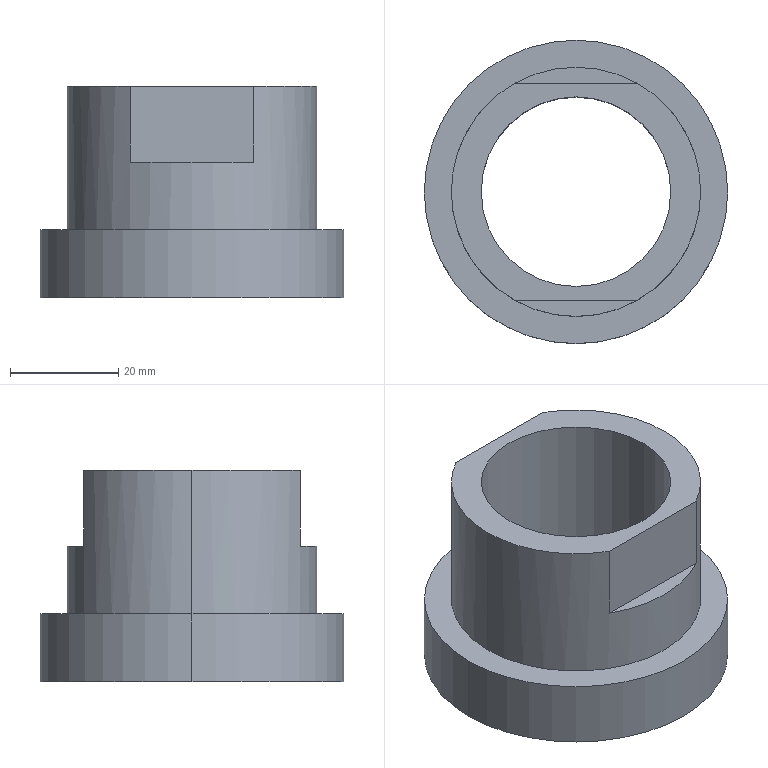Part | STEP file | DAU NOI XY LANH 125 | 1 solid | 13 faces | box 56 x 56 x 39 mm | volume 36016 mm3 | plane 7 | cylinder 6 | commonest cylinder face diameters 35 x2 46 x2 56 x2
STEP:
#1=CARTESIAN_POINT('',(0.,0.,0.));
#2=DIRECTION('',(0.,0.,1.));
#3=DIRECTION('',(1.,0.,0.));
#4=AXIS2_PLACEMENT_3D('',#1,#2,#3);
#5=CARTESIAN_POINT('',(-17.5,0.,39.));
#6=VERTEX_POINT('',#5);
#7=CARTESIAN_POINT('',(-17.5,0.,0.));
#8=VERTEX_POINT('',#7);
#9=CARTESIAN_POINT('',(-17.5,0.,39.));
#10=DIRECTION('',(0.,0.,-1.));
#11=VECTOR('',#10,1.);
#12=LINE('',#9,#11);
#13=CARTESIAN_POINT('',(0.,0.,39.));
#14=DIRECTION('',(0.,0.,-1.));
#15=DIRECTION('',(-1.,0.,0.));
#16=AXIS2_PLACEMENT_3D('',#13,#14,#15);
#17=CYLINDRICAL_SURFACE('',#16,17.5);
#18=CARTESIAN_POINT('',(6.283,0.));
#19=DIRECTION('',(0.,1.));
#20=VECTOR('',#19,1.);
#21=LINE('',#18,#20);
#22=(GEOMETRIC_REPRESENTATION_CONTEXT(2)PARAMETRIC_REPRESENTATION_CONTEXT()REPRESENTATION_CONTEXT('',''));
#23=DEFINITIONAL_REPRESENTATION('',(#21),#22);
#24=PCURVE('',#17,#23);
#25=CARTESIAN_POINT('',(0.,0.,39.));
#26=DIRECTION('',(0.,0.,-1.));
#27=DIRECTION('',(-1.,0.,0.));
#28=AXIS2_PLACEMENT_3D('',#25,#26,#27);
#29=CYLINDRICAL_SURFACE('',#28,17.5);
#30=CARTESIAN_POINT('',(0.,0.));
#31=DIRECTION('',(0.,1.));
#32=VECTOR('',#31,1.);
#33=LINE('',#30,#32);
#34=(GEOMETRIC_REPRESENTATION_CONTEXT(2)PARAMETRIC_REPRESENTATION_CONTEXT()REPRESENTATION_CONTEXT('',''));
#35=DEFINITIONAL_REPRESENTATION('',(#33),#34);
#36=PCURVE('',#29,#35);
#37=SURFACE_CURVE('',#12,(#24,#36),.PCURVE_S1.);
#38=EDGE_CURVE('',#6,#8,#37,.T.);
#39=ORIENTED_EDGE('',*,*,#38,.T.);
#40=CARTESIAN_POINT('',(17.5,0.,0.));
#41=VERTEX_POINT('',#40);
#42=CARTESIAN_POINT('',(0.,0.,0.));
#43=DIRECTION('',(0.,0.,1.));
#44=DIRECTION('',(-1.,0.,0.));
#45=AXIS2_PLACEMENT_3D('',#42,#43,#44);
#46=CIRCLE('',#45,17.5);
#47=CARTESIAN_POINT('',(6.283,39.));
#48=DIRECTION('',(-1.,0.));
#49=VECTOR('',#48,1.);
#50=LINE('',#47,#49);
#51=(GEOMETRIC_REPRESENTATION_CONTEXT(2)PARAMETRIC_REPRESENTATION_CONTEXT()REPRESENTATION_CONTEXT('',''));
#52=DEFINITIONAL_REPRESENTATION('',(#50),#51);
#53=PCURVE('',#17,#52);
#54=CARTESIAN_POINT('',(0.,0.,0.));
#55=DIRECTION('',(0.,0.,-1.));
#56=DIRECTION('',(-1.,0.,0.));
#57=AXIS2_PLACEMENT_3D('',#54,#55,#56);
#58=PLANE('',#57);
#59=CARTESIAN_POINT('',(17.5,0.));
#60=CARTESIAN_POINT('',(17.5,-30.311));
#61=CARTESIAN_POINT('',(-8.75,-15.155));
#62=CARTESIAN_POINT('',(-35.,0.));
#63=CARTESIAN_POINT('',(-8.75,15.155));
#64=CARTESIAN_POINT('',(17.5,30.311));
#65=CARTESIAN_POINT('',(17.5,0.));
#66=(BOUNDED_CURVE()B_SPLINE_CURVE(2,(#59,#60,#61,#62,#63,#64,#65),.UNSPECIFIED.,.T.,.F.)B_SPLINE_CURVE_WITH_KNOTS((1,2,2,2,2,1),(-2.094,0.,2.094,4.189,6.283,8.378),.UNSPECIFIED.)CURVE()GEOMETRIC_REPRESENTATION_ITEM()RATIONAL_B_SPLINE_CURVE((1.,0.5,1.,0.5,1.,0.5,1.))REPRESENTATION_ITEM(''));
#67=(GEOMETRIC_REPRESENTATION_CONTEXT(2)PARAMETRIC_REPRESENTATION_CONTEXT()REPRESENTATION_CONTEXT('',''));
#68=DEFINITIONAL_REPRESENTATION('',(#66),#67);
#69=PCURVE('',#58,#68);
#70=SURFACE_CURVE('',#46,(#53,#69),.PCURVE_S1.);
#71=EDGE_CURVE('',#8,#41,#70,.T.);
#72=ORIENTED_EDGE('',*,*,#71,.T.);
#73=CARTESIAN_POINT('',(17.5,0.,39.));
#74=VERTEX_POINT('',#73);
#75=CARTESIAN_POINT('',(17.5,0.,39.));
#76=DIRECTION('',(0.,0.,-1.));
#77=VECTOR('',#76,1.);
#78=LINE('',#75,#77);
#79=CARTESIAN_POINT('',(3.142,0.));
#80=DIRECTION('',(0.,1.));
#81=VECTOR('',#80,1.);
#82=LINE('',#79,#81);
#83=(GEOMETRIC_REPRESENTATION_CONTEXT(2)PARAMETRIC_REPRESENTATION_CONTEXT()REPRESENTATION_CONTEXT('',''));
#84=DEFINITIONAL_REPRESENTATION('',(#82),#83);
#85=PCURVE('',#17,#84);
#86=CARTESIAN_POINT('',(3.142,0.));
#87=DIRECTION('',(0.,1.));
#88=VECTOR('',#87,1.);
#89=LINE('',#86,#88);
#90=(GEOMETRIC_REPRESENTATION_CONTEXT(2)PARAMETRIC_REPRESENTATION_CONTEXT()REPRESENTATION_CONTEXT('',''));
#91=DEFINITIONAL_REPRESENTATION('',(#89),#90);
#92=PCURVE('',#29,#91);
#93=SURFACE_CURVE('',#78,(#85,#92),.PCURVE_S1.);
#94=EDGE_CURVE('',#74,#41,#93,.T.);
#95=ORIENTED_EDGE('',*,*,#94,.F.);
#96=CARTESIAN_POINT('',(0.,0.,39.));
#97=DIRECTION('',(0.,0.,-1.));
#98=DIRECTION('',(-1.,0.,0.));
#99=AXIS2_PLACEMENT_3D('',#96,#97,#98);
#100=CIRCLE('',#99,17.5);
#101=CARTESIAN_POINT('',(0.,0.));
#102=DIRECTION('',(1.,0.));
#103=VECTOR('',#102,1.);
#104=LINE('',#101,#103);
#105=(GEOMETRIC_REPRESENTATION_CONTEXT(2)PARAMETRIC_REPRESENTATION_CONTEXT()REPRESENTATION_CONTEXT('',''));
#106=DEFINITIONAL_REPRESENTATION('',(#104),#105);
#107=PCURVE('',#17,#106);
#108=CARTESIAN_POINT('',(0.,0.,39.));
#109=DIRECTION('',(0.,0.,-1.));
#110=DIRECTION('',(-1.,0.,0.));
#111=AXIS2_PLACEMENT_3D('',#108,#109,#110);
#112=PLANE('',#111);
#113=CARTESIAN_POINT('',(0.,0.));
#114=DIRECTION('',(1.,0.));
#115=AXIS2_PLACEMENT_2D('',#113,#114);
#116=CIRCLE('',#115,17.5);
#117=(GEOMETRIC_REPRESENTATION_CONTEXT(2)PARAMETRIC_REPRESENTATION_CONTEXT()REPRESENTATION_CONTEXT('',''));
#118=DEFINITIONAL_REPRESENTATION('',(#116),#117);
#119=PCURVE('',#112,#118);
#120=SURFACE_CURVE('',#100,(#107,#119),.PCURVE_S1.);
#121=EDGE_CURVE('',#74,#6,#120,.T.);
#122=ORIENTED_EDGE('',*,*,#121,.T.);
#123=EDGE_LOOP('',(#39,#72,#95,#122));
#124=FACE_BOUND('',#123,.F.);
#125=ADVANCED_FACE('',(#124),#17,.F.);
#126=CARTESIAN_POINT('',(23.,0.,12.5));
#127=VERTEX_POINT('',#126);
#128=CARTESIAN_POINT('',(-23.,0.,12.5));
#129=VERTEX_POINT('',#128);
#130=CARTESIAN_POINT('',(0.,0.,12.5));
#131=DIRECTION('',(0.,0.,1.));
#132=DIRECTION('',(1.,0.,0.));
#133=AXIS2_PLACEMENT_3D('',#130,#131,#132);
#134=CIRCLE('',#133,23.);
#135=CARTESIAN_POINT('',(0.,0.,12.5));
#136=DIRECTION('',(0.,0.,1.));
#137=DIRECTION('',(1.,0.,0.));
#138=AXIS2_PLACEMENT_3D('',#135,#136,#137);
#139=CYLINDRICAL_SURFACE('',#138,23.);
#140=CARTESIAN_POINT('',(0.,0.));
#141=DIRECTION('',(1.,0.));
#142=VECTOR('',#141,1.);
#143=LINE('',#140,#142);
#144=(GEOMETRIC_REPRESENTATION_CONTEXT(2)PARAMETRIC_REPRESENTATION_CONTEXT()REPRESENTATION_CONTEXT('',''));
#145=DEFINITIONAL_REPRESENTATION('',(#143),#144);
#146=PCURVE('',#139,#145);
#147=CARTESIAN_POINT('',(0.,0.,12.5));
#148=DIRECTION('',(0.,0.,-1.));
#149=DIRECTION('',(-1.,0.,0.));
#150=AXIS2_PLACEMENT_3D('',#147,#148,#149);
#151=PLANE('',#150);
#152=CARTESIAN_POINT('',(-23.,0.));
#153=CARTESIAN_POINT('',(-23.,39.837));
#154=CARTESIAN_POINT('',(11.5,19.919));
#155=CARTESIAN_POINT('',(46.,0.));
#156=CARTESIAN_POINT('',(11.5,-19.919));
#157=CARTESIAN_POINT('',(-23.,-39.837));
#158=CARTESIAN_POINT('',(-23.,0.));
#159=(BOUNDED_CURVE()B_SPLINE_CURVE(2,(#152,#153,#154,#155,#156,#157,#158),.UNSPECIFIED.,.T.,.F.)B_SPLINE_CURVE_WITH_KNOTS((1,2,2,2,2,1),(-2.094,0.,2.094,4.189,6.283,8.378),.UNSPECIFIED.)CURVE()GEOMETRIC_REPRESENTATION_ITEM()RATIONAL_B_SPLINE_CURVE((1.,0.5,1.,0.5,1.,0.5,1.))REPRESENTATION_ITEM(''));
#160=(GEOMETRIC_REPRESENTATION_CONTEXT(2)PARAMETRIC_REPRESENTATION_CONTEXT()REPRESENTATION_CONTEXT('',''));
#161=DEFINITIONAL_REPRESENTATION('',(#159),#160);
#162=PCURVE('',#151,#161);
#163=SURFACE_CURVE('',#134,(#146,#162),.PCURVE_S1.);
#164=EDGE_CURVE('',#127,#129,#163,.T.);
#165=ORIENTED_EDGE('',*,*,#164,.T.);
#166=CARTESIAN_POINT('',(-23.,0.,39.));
#167=VERTEX_POINT('',#166);
#168=CARTESIAN_POINT('',(-23.,0.,12.5));
#169=DIRECTION('',(0.,0.,1.));
#170=VECTOR('',#169,1.);
#171=LINE('',#168,#170);
#172=CARTESIAN_POINT('',(3.142,0.));
#173=DIRECTION('',(0.,1.));
#174=VECTOR('',#173,1.);
#175=LINE('',#172,#174);
#176=(GEOMETRIC_REPRESENTATION_CONTEXT(2)PARAMETRIC_REPRESENTATION_CONTEXT()REPRESENTATION_CONTEXT('',''));
#177=DEFINITIONAL_REPRESENTATION('',(#175),#176);
#178=PCURVE('',#139,#177);
#179=CARTESIAN_POINT('',(0.,0.,12.5));
#180=DIRECTION('',(0.,0.,1.));
#181=DIRECTION('',(1.,0.,0.));
#182=AXIS2_PLACEMENT_3D('',#179,#180,#181);
#183=CYLINDRICAL_SURFACE('',#182,23.);
#184=CARTESIAN_POINT('',(3.142,0.));
#185=DIRECTION('',(0.,1.));
#186=VECTOR('',#185,1.);
#187=LINE('',#184,#186);
#188=(GEOMETRIC_REPRESENTATION_CONTEXT(2)PARAMETRIC_REPRESENTATION_CONTEXT()REPRESENTATION_CONTEXT('',''));
#189=DEFINITIONAL_REPRESENTATION('',(#187),#188);
#190=PCURVE('',#183,#189);
#191=SURFACE_CURVE('',#171,(#178,#190),.PCURVE_S1.);
#192=EDGE_CURVE('',#129,#167,#191,.T.);
#193=ORIENTED_EDGE('',*,*,#192,.T.);
#194=CARTESIAN_POINT('',(-11.358,20.,39.));
#195=VERTEX_POINT('',#194);
#196=CARTESIAN_POINT('',(0.,0.,39.));
#197=DIRECTION('',(0.,0.,-1.));
#198=DIRECTION('',(1.,0.,0.));
#199=AXIS2_PLACEMENT_3D('',#196,#197,#198);
#200=CIRCLE('',#199,23.);
#201=CARTESIAN_POINT('',(6.283,26.5));
#202=DIRECTION('',(-1.,0.));
#203=VECTOR('',#202,1.);
#204=LINE('',#201,#203);
#205=(GEOMETRIC_REPRESENTATION_CONTEXT(2)PARAMETRIC_REPRESENTATION_CONTEXT()REPRESENTATION_CONTEXT('',''));
#206=DEFINITIONAL_REPRESENTATION('',(#204),#205);
#207=PCURVE('',#139,#206);
#208=CARTESIAN_POINT('',(0.,0.));
#209=DIRECTION('',(-1.,0.));
#210=AXIS2_PLACEMENT_2D('',#208,#209);
#211=CIRCLE('',#210,23.);
#212=(GEOMETRIC_REPRESENTATION_CONTEXT(2)PARAMETRIC_REPRESENTATION_CONTEXT()REPRESENTATION_CONTEXT('',''));
#213=DEFINITIONAL_REPRESENTATION('',(#211),#212);
#214=PCURVE('',#112,#213);
#215=SURFACE_CURVE('',#200,(#207,#214),.PCURVE_S1.);
#216=EDGE_CURVE('',#167,#195,#215,.T.);
#217=ORIENTED_EDGE('',*,*,#216,.T.);
#218=CARTESIAN_POINT('',(-11.358,20.,25.));
#219=VERTEX_POINT('',#218);
#220=CARTESIAN_POINT('',(-11.358,20.,12.5));
#221=DIRECTION('',(0.,0.,-1.));
#222=VECTOR('',#221,1.);
#223=LINE('',#220,#222);
#224=CARTESIAN_POINT('',(2.087,0.));
#225=DIRECTION('',(0.,-1.));
#226=VECTOR('',#225,1.);
#227=LINE('',#224,#226);
#228=(GEOMETRIC_REPRESENTATION_CONTEXT(2)PARAMETRIC_REPRESENTATION_CONTEXT()REPRESENTATION_CONTEXT('',''));
#229=DEFINITIONAL_REPRESENTATION('',(#227),#228);
#230=PCURVE('',#139,#229);
#231=CARTESIAN_POINT('',(-15.,20.,39.));
#232=DIRECTION('',(0.,-1.,0.));
#233=DIRECTION('',(0.,0.,-1.));
#234=AXIS2_PLACEMENT_3D('',#231,#232,#233);
#235=PLANE('',#234);
#236=CARTESIAN_POINT('',(26.5,3.642));
#237=DIRECTION('',(1.,0.));
#238=VECTOR('',#237,1.);
#239=LINE('',#236,#238);
#240=(GEOMETRIC_REPRESENTATION_CONTEXT(2)PARAMETRIC_REPRESENTATION_CONTEXT()REPRESENTATION_CONTEXT('',''));
#241=DEFINITIONAL_REPRESENTATION('',(#239),#240);
#242=PCURVE('',#235,#241);
#243=SURFACE_CURVE('',#223,(#230,#242),.PCURVE_S1.);
#244=EDGE_CURVE('',#195,#219,#243,.T.);
#245=ORIENTED_EDGE('',*,*,#244,.T.);
#246=CARTESIAN_POINT('',(11.358,20.,25.));
#247=VERTEX_POINT('',#246);
#248=CARTESIAN_POINT('',(0.,0.,25.));
#249=DIRECTION('',(0.,0.,-1.));
#250=DIRECTION('',(1.,0.,0.));
#251=AXIS2_PLACEMENT_3D('',#248,#249,#250);
#252=CIRCLE('',#251,23.);
#253=CARTESIAN_POINT('',(6.283,12.5));
#254=DIRECTION('',(-1.,0.));
#255=VECTOR('',#254,1.);
#256=LINE('',#253,#255);
#257=(GEOMETRIC_REPRESENTATION_CONTEXT(2)PARAMETRIC_REPRESENTATION_CONTEXT()REPRESENTATION_CONTEXT('',''));
#258=DEFINITIONAL_REPRESENTATION('',(#256),#257);
#259=PCURVE('',#139,#258);
#260=CARTESIAN_POINT('',(0.,25.,25.));
#261=DIRECTION('',(0.,0.,1.));
#262=DIRECTION('',(1.,0.,0.));
#263=AXIS2_PLACEMENT_3D('',#260,#261,#262);
#264=PLANE('',#263);
#265=CARTESIAN_POINT('',(23.,-25.));
#266=CARTESIAN_POINT('',(23.,-64.837));
#267=CARTESIAN_POINT('',(-11.5,-44.919));
#268=CARTESIAN_POINT('',(-46.,-25.));
#269=CARTESIAN_POINT('',(-11.5,-5.081));
#270=CARTESIAN_POINT('',(23.,14.837));
#271=CARTESIAN_POINT('',(23.,-25.));
#272=(BOUNDED_CURVE()B_SPLINE_CURVE(2,(#265,#266,#267,#268,#269,#270,#271),.UNSPECIFIED.,.T.,.F.)B_SPLINE_CURVE_WITH_KNOTS((1,2,2,2,2,1),(-2.094,0.,2.094,4.189,6.283,8.378),.UNSPECIFIED.)CURVE()GEOMETRIC_REPRESENTATION_ITEM()RATIONAL_B_SPLINE_CURVE((1.,0.5,1.,0.5,1.,0.5,1.))REPRESENTATION_ITEM(''));
#273=(GEOMETRIC_REPRESENTATION_CONTEXT(2)PARAMETRIC_REPRESENTATION_CONTEXT()REPRESENTATION_CONTEXT('',''));
#274=DEFINITIONAL_REPRESENTATION('',(#272),#273);
#275=PCURVE('',#264,#274);
#276=SURFACE_CURVE('',#252,(#259,#275),.PCURVE_S1.);
#277=EDGE_CURVE('',#219,#247,#276,.T.);
#278=ORIENTED_EDGE('',*,*,#277,.T.);
#279=CARTESIAN_POINT('',(11.358,20.,39.));
#280=VERTEX_POINT('',#279);
#281=CARTESIAN_POINT('',(11.358,20.,12.5));
#282=DIRECTION('',(0.,0.,1.));
#283=VECTOR('',#282,1.);
#284=LINE('',#281,#283);
#285=CARTESIAN_POINT('',(1.054,0.));
#286=DIRECTION('',(0.,1.));
#287=VECTOR('',#286,1.);
#288=LINE('',#285,#287);
#289=(GEOMETRIC_REPRESENTATION_CONTEXT(2)PARAMETRIC_REPRESENTATION_CONTEXT()REPRESENTATION_CONTEXT('',''));
#290=DEFINITIONAL_REPRESENTATION('',(#288),#289);
#291=PCURVE('',#139,#290);
#292=CARTESIAN_POINT('',(26.5,26.358));
#293=DIRECTION('',(-1.,0.));
#294=VECTOR('',#293,1.);
#295=LINE('',#292,#294);
#296=(GEOMETRIC_REPRESENTATION_CONTEXT(2)PARAMETRIC_REPRESENTATION_CONTEXT()REPRESENTATION_CONTEXT('',''));
#297=DEFINITIONAL_REPRESENTATION('',(#295),#296);
#298=PCURVE('',#235,#297);
#299=SURFACE_CURVE('',#284,(#291,#298),.PCURVE_S1.);
#300=EDGE_CURVE('',#247,#280,#299,.T.);
#301=ORIENTED_EDGE('',*,*,#300,.T.);
#302=CARTESIAN_POINT('',(23.,0.,39.));
#303=VERTEX_POINT('',#302);
#304=CARTESIAN_POINT('',(0.,0.,39.));
#305=DIRECTION('',(0.,0.,-1.));
#306=DIRECTION('',(1.,0.,0.));
#307=AXIS2_PLACEMENT_3D('',#304,#305,#306);
#308=CIRCLE('',#307,23.);
#309=CARTESIAN_POINT('',(6.283,26.5));
#310=DIRECTION('',(-1.,0.));
#311=VECTOR('',#310,1.);
#312=LINE('',#309,#311);
#313=(GEOMETRIC_REPRESENTATION_CONTEXT(2)PARAMETRIC_REPRESENTATION_CONTEXT()REPRESENTATION_CONTEXT('',''));
#314=DEFINITIONAL_REPRESENTATION('',(#312),#313);
#315=PCURVE('',#139,#314);
#316=CARTESIAN_POINT('',(0.,0.));
#317=DIRECTION('',(-1.,0.));
#318=AXIS2_PLACEMENT_2D('',#316,#317);
#319=CIRCLE('',#318,23.);
#320=(GEOMETRIC_REPRESENTATION_CONTEXT(2)PARAMETRIC_REPRESENTATION_CONTEXT()REPRESENTATION_CONTEXT('',''));
#321=DEFINITIONAL_REPRESENTATION('',(#319),#320);
#322=PCURVE('',#112,#321);
#323=SURFACE_CURVE('',#308,(#315,#322),.PCURVE_S1.);
#324=EDGE_CURVE('',#280,#303,#323,.T.);
#325=ORIENTED_EDGE('',*,*,#324,.T.);
#326=CARTESIAN_POINT('',(23.,0.,12.5));
#327=DIRECTION('',(0.,0.,1.));
#328=VECTOR('',#327,1.);
#329=LINE('',#326,#328);
#330=CARTESIAN_POINT('',(0.,0.));
#331=DIRECTION('',(0.,1.));
#332=VECTOR('',#331,1.);
#333=LINE('',#330,#332);
#334=(GEOMETRIC_REPRESENTATION_CONTEXT(2)PARAMETRIC_REPRESENTATION_CONTEXT()REPRESENTATION_CONTEXT('',''));
#335=DEFINITIONAL_REPRESENTATION('',(#333),#334);
#336=PCURVE('',#139,#335);
#337=CARTESIAN_POINT('',(6.283,0.));
#338=DIRECTION('',(0.,1.));
#339=VECTOR('',#338,1.);
#340=LINE('',#337,#339);
#341=(GEOMETRIC_REPRESENTATION_CONTEXT(2)PARAMETRIC_REPRESENTATION_CONTEXT()REPRESENTATION_CONTEXT('',''));
#342=DEFINITIONAL_REPRESENTATION('',(#340),#341);
#343=PCURVE('',#183,#342);
#344=SURFACE_CURVE('',#329,(#336,#343),.PCURVE_S1.);
#345=EDGE_CURVE('',#127,#303,#344,.T.);
#346=ORIENTED_EDGE('',*,*,#345,.F.);
#347=EDGE_LOOP('',(#165,#193,#217,#245,#278,#301,#325,#346));
#348=FACE_BOUND('',#347,.T.);
#349=ADVANCED_FACE('',(#348),#139,.T.);
#350=CARTESIAN_POINT('',(-28.,0.,0.));
#351=VERTEX_POINT('',#350);
#352=CARTESIAN_POINT('',(28.,0.,0.));
#353=VERTEX_POINT('',#352);
#354=CARTESIAN_POINT('',(0.,0.,0.));
#355=DIRECTION('',(0.,0.,-1.));
#356=DIRECTION('',(1.,0.,0.));
#357=AXIS2_PLACEMENT_3D('',#354,#355,#356);
#358=CIRCLE('',#357,28.);
#359=CARTESIAN_POINT('',(0.,0.,0.));
#360=DIRECTION('',(0.,0.,1.));
#361=DIRECTION('',(1.,0.,0.));
#362=AXIS2_PLACEMENT_3D('',#359,#360,#361);
#363=CYLINDRICAL_SURFACE('',#362,28.);
#364=CARTESIAN_POINT('',(6.283,0.));
#365=DIRECTION('',(-1.,0.));
#366=VECTOR('',#365,1.);
#367=LINE('',#364,#366);
#368=(GEOMETRIC_REPRESENTATION_CONTEXT(2)PARAMETRIC_REPRESENTATION_CONTEXT()REPRESENTATION_CONTEXT('',''));
#369=DEFINITIONAL_REPRESENTATION('',(#367),#368);
#370=PCURVE('',#363,#369);
#371=CARTESIAN_POINT('',(0.,0.));
#372=DIRECTION('',(-1.,0.));
#373=AXIS2_PLACEMENT_2D('',#371,#372);
#374=CIRCLE('',#373,28.);
#375=(GEOMETRIC_REPRESENTATION_CONTEXT(2)PARAMETRIC_REPRESENTATION_CONTEXT()REPRESENTATION_CONTEXT('',''));
#376=DEFINITIONAL_REPRESENTATION('',(#374),#375);
#377=PCURVE('',#58,#376);
#378=SURFACE_CURVE('',#358,(#370,#377),.PCURVE_S1.);
#379=EDGE_CURVE('',#351,#353,#378,.T.);
#380=ORIENTED_EDGE('',*,*,#379,.F.);
#381=CARTESIAN_POINT('',(-28.,0.,12.5));
#382=VERTEX_POINT('',#381);
#383=CARTESIAN_POINT('',(-28.,0.,0.));
#384=DIRECTION('',(0.,0.,1.));
#385=VECTOR('',#384,1.);
#386=LINE('',#383,#385);
#387=CARTESIAN_POINT('',(3.142,0.));
#388=DIRECTION('',(0.,1.));
#389=VECTOR('',#388,1.);
#390=LINE('',#387,#389);
#391=(GEOMETRIC_REPRESENTATION_CONTEXT(2)PARAMETRIC_REPRESENTATION_CONTEXT()REPRESENTATION_CONTEXT('',''));
#392=DEFINITIONAL_REPRESENTATION('',(#390),#391);
#393=PCURVE('',#363,#392);
#394=CARTESIAN_POINT('',(0.,0.,0.));
#395=DIRECTION('',(0.,0.,1.));
#396=DIRECTION('',(1.,0.,0.));
#397=AXIS2_PLACEMENT_3D('',#394,#395,#396);
#398=CYLINDRICAL_SURFACE('',#397,28.);
#399=CARTESIAN_POINT('',(3.142,0.));
#400=DIRECTION('',(0.,1.));
#401=VECTOR('',#400,1.);
#402=LINE('',#399,#401);
#403=(GEOMETRIC_REPRESENTATION_CONTEXT(2)PARAMETRIC_REPRESENTATION_CONTEXT()REPRESENTATION_CONTEXT('',''));
#404=DEFINITIONAL_REPRESENTATION('',(#402),#403);
#405=PCURVE('',#398,#404);
#406=SURFACE_CURVE('',#386,(#393,#405),.PCURVE_S1.);
#407=EDGE_CURVE('',#351,#382,#406,.T.);
#408=ORIENTED_EDGE('',*,*,#407,.T.);
#409=CARTESIAN_POINT('',(28.,0.,12.5));
#410=VERTEX_POINT('',#409);
#411=CARTESIAN_POINT('',(0.,0.,12.5));
#412=DIRECTION('',(0.,0.,-1.));
#413=DIRECTION('',(1.,0.,0.));
#414=AXIS2_PLACEMENT_3D('',#411,#412,#413);
#415=CIRCLE('',#414,28.);
#416=CARTESIAN_POINT('',(6.283,12.5));
#417=DIRECTION('',(-1.,0.));
#418=VECTOR('',#417,1.);
#419=LINE('',#416,#418);
#420=(GEOMETRIC_REPRESENTATION_CONTEXT(2)PARAMETRIC_REPRESENTATION_CONTEXT()REPRESENTATION_CONTEXT('',''));
#421=DEFINITIONAL_REPRESENTATION('',(#419),#420);
#422=PCURVE('',#363,#421);
#423=CARTESIAN_POINT('',(0.,0.));
#424=DIRECTION('',(-1.,0.));
#425=AXIS2_PLACEMENT_2D('',#423,#424);
#426=CIRCLE('',#425,28.);
#427=(GEOMETRIC_REPRESENTATION_CONTEXT(2)PARAMETRIC_REPRESENTATION_CONTEXT()REPRESENTATION_CONTEXT('',''));
#428=DEFINITIONAL_REPRESENTATION('',(#426),#427);
#429=PCURVE('',#151,#428);
#430=SURFACE_CURVE('',#415,(#422,#429),.PCURVE_S1.);
#431=EDGE_CURVE('',#382,#410,#430,.T.);
#432=ORIENTED_EDGE('',*,*,#431,.T.);
#433=CARTESIAN_POINT('',(28.,0.,0.));
#434=DIRECTION('',(0.,0.,1.));
#435=VECTOR('',#434,1.);
#436=LINE('',#433,#435);
#437=CARTESIAN_POINT('',(0.,0.));
#438=DIRECTION('',(0.,1.));
#439=VECTOR('',#438,1.);
#440=LINE('',#437,#439);
#441=(GEOMETRIC_REPRESENTATION_CONTEXT(2)PARAMETRIC_REPRESENTATION_CONTEXT()REPRESENTATION_CONTEXT('',''));
#442=DEFINITIONAL_REPRESENTATION('',(#440),#441);
#443=PCURVE('',#363,#442);
#444=CARTESIAN_POINT('',(6.283,0.));
#445=DIRECTION('',(0.,1.));
#446=VECTOR('',#445,1.);
#447=LINE('',#444,#446);
#448=(GEOMETRIC_REPRESENTATION_CONTEXT(2)PARAMETRIC_REPRESENTATION_CONTEXT()REPRESENTATION_CONTEXT('',''));
#449=DEFINITIONAL_REPRESENTATION('',(#447),#448);
#450=PCURVE('',#398,#449);
#451=SURFACE_CURVE('',#436,(#443,#450),.PCURVE_S1.);
#452=EDGE_CURVE('',#353,#410,#451,.T.);
#453=ORIENTED_EDGE('',*,*,#452,.F.);
#454=EDGE_LOOP('',(#380,#408,#432,#453));
#455=FACE_BOUND('',#454,.T.);
#456=ADVANCED_FACE('',(#455),#363,.T.);
#457=CARTESIAN_POINT('',(0.,0.,0.));
#458=DIRECTION('',(0.,0.,1.));
#459=DIRECTION('',(-1.,0.,0.));
#460=AXIS2_PLACEMENT_3D('',#457,#458,#459);
#461=CIRCLE('',#460,17.5);
#462=CARTESIAN_POINT('',(6.283,39.));
#463=DIRECTION('',(-1.,0.));
#464=VECTOR('',#463,1.);
#465=LINE('',#462,#464);
#466=(GEOMETRIC_REPRESENTATION_CONTEXT(2)PARAMETRIC_REPRESENTATION_CONTEXT()REPRESENTATION_CONTEXT('',''));
#467=DEFINITIONAL_REPRESENTATION('',(#465),#466);
#468=PCURVE('',#29,#467);
#469=CARTESIAN_POINT('',(17.5,0.));
#470=CARTESIAN_POINT('',(17.5,-30.311));
#471=CARTESIAN_POINT('',(-8.75,-15.155));
#472=CARTESIAN_POINT('',(-35.,0.));
#473=CARTESIAN_POINT('',(-8.75,15.155));
#474=CARTESIAN_POINT('',(17.5,30.311));
#475=CARTESIAN_POINT('',(17.5,0.));
#476=(BOUNDED_CURVE()B_SPLINE_CURVE(2,(#469,#470,#471,#472,#473,#474,#475),.UNSPECIFIED.,.T.,.F.)B_SPLINE_CURVE_WITH_KNOTS((1,2,2,2,2,1),(-2.094,0.,2.094,4.189,6.283,8.378),.UNSPECIFIED.)CURVE()GEOMETRIC_REPRESENTATION_ITEM()RATIONAL_B_SPLINE_CURVE((1.,0.5,1.,0.5,1.,0.5,1.))REPRESENTATION_ITEM(''));
#477=(GEOMETRIC_REPRESENTATION_CONTEXT(2)PARAMETRIC_REPRESENTATION_CONTEXT()REPRESENTATION_CONTEXT('',''));
#478=DEFINITIONAL_REPRESENTATION('',(#476),#477);
#479=PCURVE('',#58,#478);
#480=SURFACE_CURVE('',#461,(#468,#479),.PCURVE_S1.);
#481=EDGE_CURVE('',#41,#8,#480,.T.);
#482=ORIENTED_EDGE('',*,*,#481,.T.);
#483=ORIENTED_EDGE('',*,*,#38,.F.);
#484=CARTESIAN_POINT('',(0.,0.,39.));
#485=DIRECTION('',(0.,0.,-1.));
#486=DIRECTION('',(-1.,0.,0.));
#487=AXIS2_PLACEMENT_3D('',#484,#485,#486);
#488=CIRCLE('',#487,17.5);
#489=CARTESIAN_POINT('',(0.,0.));
#490=DIRECTION('',(1.,0.));
#491=VECTOR('',#490,1.);
#492=LINE('',#489,#491);
#493=(GEOMETRIC_REPRESENTATION_CONTEXT(2)PARAMETRIC_REPRESENTATION_CONTEXT()REPRESENTATION_CONTEXT('',''));
#494=DEFINITIONAL_REPRESENTATION('',(#492),#493);
#495=PCURVE('',#29,#494);
#496=CARTESIAN_POINT('',(0.,0.));
#497=DIRECTION('',(1.,0.));
#498=AXIS2_PLACEMENT_2D('',#496,#497);
#499=CIRCLE('',#498,17.5);
#500=(GEOMETRIC_REPRESENTATION_CONTEXT(2)PARAMETRIC_REPRESENTATION_CONTEXT()REPRESENTATION_CONTEXT('',''));
#501=DEFINITIONAL_REPRESENTATION('',(#499),#500);
#502=PCURVE('',#112,#501);
#503=SURFACE_CURVE('',#488,(#495,#502),.PCURVE_S1.);
#504=EDGE_CURVE('',#6,#74,#503,.T.);
#505=ORIENTED_EDGE('',*,*,#504,.T.);
#506=ORIENTED_EDGE('',*,*,#94,.T.);
#507=EDGE_LOOP('',(#482,#483,#505,#506));
#508=FACE_BOUND('',#507,.F.);
#509=ADVANCED_FACE('',(#508),#29,.F.);
#510=ORIENTED_EDGE('',*,*,#504,.T.);
#511=ORIENTED_EDGE('',*,*,#121,.T.);
#512=EDGE_LOOP('',(#510,#511));
#513=FACE_BOUND('',#512,.T.);
#514=ORIENTED_EDGE('',*,*,#324,.F.);
#515=CARTESIAN_POINT('',(0.,20.,39.));
#516=DIRECTION('',(1.,0.,0.));
#517=VECTOR('',#516,1.);
#518=LINE('',#515,#517);
#519=CARTESIAN_POINT('',(0.,20.));
#520=DIRECTION('',(-1.,0.));
#521=VECTOR('',#520,1.);
#522=LINE('',#519,#521);
#523=(GEOMETRIC_REPRESENTATION_CONTEXT(2)PARAMETRIC_REPRESENTATION_CONTEXT()REPRESENTATION_CONTEXT('',''));
#524=DEFINITIONAL_REPRESENTATION('',(#522),#523);
#525=PCURVE('',#112,#524);
#526=CARTESIAN_POINT('',(0.,15.));
#527=DIRECTION('',(0.,1.));
#528=VECTOR('',#527,1.);
#529=LINE('',#526,#528);
#530=(GEOMETRIC_REPRESENTATION_CONTEXT(2)PARAMETRIC_REPRESENTATION_CONTEXT()REPRESENTATION_CONTEXT('',''));
#531=DEFINITIONAL_REPRESENTATION('',(#529),#530);
#532=PCURVE('',#235,#531);
#533=SURFACE_CURVE('',#518,(#525,#532),.PCURVE_S1.);
#534=EDGE_CURVE('',#195,#280,#533,.T.);
#535=ORIENTED_EDGE('',*,*,#534,.F.);
#536=ORIENTED_EDGE('',*,*,#216,.F.);
#537=CARTESIAN_POINT('',(-11.358,-20.,39.));
#538=VERTEX_POINT('',#537);
#539=CARTESIAN_POINT('',(0.,0.,39.));
#540=DIRECTION('',(0.,0.,-1.));
#541=DIRECTION('',(1.,0.,0.));
#542=AXIS2_PLACEMENT_3D('',#539,#540,#541);
#543=CIRCLE('',#542,23.);
#544=CARTESIAN_POINT('',(0.,0.));
#545=DIRECTION('',(-1.,0.));
#546=AXIS2_PLACEMENT_2D('',#544,#545);
#547=CIRCLE('',#546,23.);
#548=(GEOMETRIC_REPRESENTATION_CONTEXT(2)PARAMETRIC_REPRESENTATION_CONTEXT()REPRESENTATION_CONTEXT('',''));
#549=DEFINITIONAL_REPRESENTATION('',(#547),#548);
#550=PCURVE('',#112,#549);
#551=CARTESIAN_POINT('',(6.283,26.5));
#552=DIRECTION('',(-1.,0.));
#553=VECTOR('',#552,1.);
#554=LINE('',#551,#553);
#555=(GEOMETRIC_REPRESENTATION_CONTEXT(2)PARAMETRIC_REPRESENTATION_CONTEXT()REPRESENTATION_CONTEXT('',''));
#556=DEFINITIONAL_REPRESENTATION('',(#554),#555);
#557=PCURVE('',#183,#556);
#558=SURFACE_CURVE('',#543,(#550,#557),.PCURVE_S1.);
#559=EDGE_CURVE('',#538,#167,#558,.T.);
#560=ORIENTED_EDGE('',*,*,#559,.F.);
#561=CARTESIAN_POINT('',(11.358,-20.,39.));
#562=VERTEX_POINT('',#561);
#563=CARTESIAN_POINT('',(0.,-20.,39.));
#564=DIRECTION('',(-1.,0.,0.));
#565=VECTOR('',#564,1.);
#566=LINE('',#563,#565);
#567=CARTESIAN_POINT('',(0.,-20.));
#568=DIRECTION('',(1.,0.));
#569=VECTOR('',#568,1.);
#570=LINE('',#567,#569);
#571=(GEOMETRIC_REPRESENTATION_CONTEXT(2)PARAMETRIC_REPRESENTATION_CONTEXT()REPRESENTATION_CONTEXT('',''));
#572=DEFINITIONAL_REPRESENTATION('',(#570),#571);
#573=PCURVE('',#112,#572);
#574=CARTESIAN_POINT('',(15.,-20.,39.));
#575=DIRECTION('',(0.,1.,0.));
#576=DIRECTION('',(0.,0.,1.));
#577=AXIS2_PLACEMENT_3D('',#574,#575,#576);
#578=PLANE('',#577);
#579=CARTESIAN_POINT('',(0.,-15.));
#580=DIRECTION('',(0.,-1.));
#581=VECTOR('',#580,1.);
#582=LINE('',#579,#581);
#583=(GEOMETRIC_REPRESENTATION_CONTEXT(2)PARAMETRIC_REPRESENTATION_CONTEXT()REPRESENTATION_CONTEXT('',''));
#584=DEFINITIONAL_REPRESENTATION('',(#582),#583);
#585=PCURVE('',#578,#584);
#586=SURFACE_CURVE('',#566,(#573,#585),.PCURVE_S1.);
#587=EDGE_CURVE('',#562,#538,#586,.T.);
#588=ORIENTED_EDGE('',*,*,#587,.F.);
#589=CARTESIAN_POINT('',(0.,0.,39.));
#590=DIRECTION('',(0.,0.,-1.));
#591=DIRECTION('',(1.,0.,0.));
#592=AXIS2_PLACEMENT_3D('',#589,#590,#591);
#593=CIRCLE('',#592,23.);
#594=CARTESIAN_POINT('',(0.,0.));
#595=DIRECTION('',(-1.,0.));
#596=AXIS2_PLACEMENT_2D('',#594,#595);
#597=CIRCLE('',#596,23.);
#598=(GEOMETRIC_REPRESENTATION_CONTEXT(2)PARAMETRIC_REPRESENTATION_CONTEXT()REPRESENTATION_CONTEXT('',''));
#599=DEFINITIONAL_REPRESENTATION('',(#597),#598);
#600=PCURVE('',#112,#599);
#601=CARTESIAN_POINT('',(6.283,26.5));
#602=DIRECTION('',(-1.,0.));
#603=VECTOR('',#602,1.);
#604=LINE('',#601,#603);
#605=(GEOMETRIC_REPRESENTATION_CONTEXT(2)PARAMETRIC_REPRESENTATION_CONTEXT()REPRESENTATION_CONTEXT('',''));
#606=DEFINITIONAL_REPRESENTATION('',(#604),#605);
#607=PCURVE('',#183,#606);
#608=SURFACE_CURVE('',#593,(#600,#607),.PCURVE_S1.);
#609=EDGE_CURVE('',#303,#562,#608,.T.);
#610=ORIENTED_EDGE('',*,*,#609,.F.);
#611=EDGE_LOOP('',(#514,#535,#536,#560,#588,#610));
#612=FACE_BOUND('',#611,.T.);
#613=ADVANCED_FACE('',(#513,#612),#112,.F.);
#614=ORIENTED_EDGE('',*,*,#71,.T.);
#615=ORIENTED_EDGE('',*,*,#481,.T.);
#616=EDGE_LOOP('',(#614,#615));
#617=FACE_BOUND('',#616,.T.);
#618=CARTESIAN_POINT('',(0.,0.,0.));
#619=DIRECTION('',(0.,0.,-1.));
#620=DIRECTION('',(1.,0.,0.));
#621=AXIS2_PLACEMENT_3D('',#618,#619,#620);
#622=CIRCLE('',#621,28.);
#623=CARTESIAN_POINT('',(0.,0.));
#624=DIRECTION('',(-1.,0.));
#625=AXIS2_PLACEMENT_2D('',#623,#624);
#626=CIRCLE('',#625,28.);
#627=(GEOMETRIC_REPRESENTATION_CONTEXT(2)PARAMETRIC_REPRESENTATION_CONTEXT()REPRESENTATION_CONTEXT('',''));
#628=DEFINITIONAL_REPRESENTATION('',(#626),#627);
#629=PCURVE('',#58,#628);
#630=CARTESIAN_POINT('',(6.283,0.));
#631=DIRECTION('',(-1.,0.));
#632=VECTOR('',#631,1.);
#633=LINE('',#630,#632);
#634=(GEOMETRIC_REPRESENTATION_CONTEXT(2)PARAMETRIC_REPRESENTATION_CONTEXT()REPRESENTATION_CONTEXT('',''));
#635=DEFINITIONAL_REPRESENTATION('',(#633),#634);
#636=PCURVE('',#398,#635);
#637=SURFACE_CURVE('',#622,(#629,#636),.PCURVE_S1.);
#638=EDGE_CURVE('',#353,#351,#637,.T.);
#639=ORIENTED_EDGE('',*,*,#638,.T.);
#640=ORIENTED_EDGE('',*,*,#379,.T.);
#641=EDGE_LOOP('',(#639,#640));
#642=FACE_BOUND('',#641,.T.);
#643=ADVANCED_FACE('',(#617,#642),#58,.T.);
#644=ORIENTED_EDGE('',*,*,#587,.T.);
#645=CARTESIAN_POINT('',(-11.358,-20.,25.));
#646=VERTEX_POINT('',#645);
#647=CARTESIAN_POINT('',(-11.358,-20.,39.));
#648=DIRECTION('',(0.,0.,1.));
#649=VECTOR('',#648,1.);
#650=LINE('',#647,#649);
#651=CARTESIAN_POINT('',(0.,-26.358));
#652=DIRECTION('',(1.,0.));
#653=VECTOR('',#652,1.);
#654=LINE('',#651,#653);
#655=(GEOMETRIC_REPRESENTATION_CONTEXT(2)PARAMETRIC_REPRESENTATION_CONTEXT()REPRESENTATION_CONTEXT('',''));
#656=DEFINITIONAL_REPRESENTATION('',(#654),#655);
#657=PCURVE('',#578,#656);
#658=CARTESIAN_POINT('',(4.196,26.5));
#659=DIRECTION('',(0.,1.));
#660=VECTOR('',#659,1.);
#661=LINE('',#658,#660);
#662=(GEOMETRIC_REPRESENTATION_CONTEXT(2)PARAMETRIC_REPRESENTATION_CONTEXT()REPRESENTATION_CONTEXT('',''));
#663=DEFINITIONAL_REPRESENTATION('',(#661),#662);
#664=PCURVE('',#183,#663);
#665=SURFACE_CURVE('',#650,(#657,#664),.PCURVE_S1.);
#666=EDGE_CURVE('',#646,#538,#665,.T.);
#667=ORIENTED_EDGE('',*,*,#666,.F.);
#668=CARTESIAN_POINT('',(11.358,-20.,25.));
#669=VERTEX_POINT('',#668);
#670=CARTESIAN_POINT('',(15.,-20.,25.));
#671=DIRECTION('',(-1.,0.,0.));
#672=VECTOR('',#671,1.);
#673=LINE('',#670,#672);
#674=CARTESIAN_POINT('',(-14.,0.));
#675=DIRECTION('',(0.,-1.));
#676=VECTOR('',#675,1.);
#677=LINE('',#674,#676);
#678=(GEOMETRIC_REPRESENTATION_CONTEXT(2)PARAMETRIC_REPRESENTATION_CONTEXT()REPRESENTATION_CONTEXT('',''));
#679=DEFINITIONAL_REPRESENTATION('',(#677),#678);
#680=PCURVE('',#578,#679);
#681=CARTESIAN_POINT('',(0.,-25.,25.));
#682=DIRECTION('',(0.,0.,1.));
#683=DIRECTION('',(1.,0.,0.));
#684=AXIS2_PLACEMENT_3D('',#681,#682,#683);
#685=PLANE('',#684);
#686=CARTESIAN_POINT('',(15.,5.));
#687=DIRECTION('',(-1.,0.));
#688=VECTOR('',#687,1.);
#689=LINE('',#686,#688);
#690=(GEOMETRIC_REPRESENTATION_CONTEXT(2)PARAMETRIC_REPRESENTATION_CONTEXT()REPRESENTATION_CONTEXT('',''));
#691=DEFINITIONAL_REPRESENTATION('',(#689),#690);
#692=PCURVE('',#685,#691);
#693=SURFACE_CURVE('',#673,(#680,#692),.PCURVE_S1.);
#694=EDGE_CURVE('',#669,#646,#693,.T.);
#695=ORIENTED_EDGE('',*,*,#694,.F.);
#696=CARTESIAN_POINT('',(11.358,-20.,39.));
#697=DIRECTION('',(0.,0.,-1.));
#698=VECTOR('',#697,1.);
#699=LINE('',#696,#698);
#700=CARTESIAN_POINT('',(0.,-3.642));
#701=DIRECTION('',(-1.,0.));
#702=VECTOR('',#701,1.);
#703=LINE('',#700,#702);
#704=(GEOMETRIC_REPRESENTATION_CONTEXT(2)PARAMETRIC_REPRESENTATION_CONTEXT()REPRESENTATION_CONTEXT('',''));
#705=DEFINITIONAL_REPRESENTATION('',(#703),#704);
#706=PCURVE('',#578,#705);
#707=CARTESIAN_POINT('',(5.229,26.5));
#708=DIRECTION('',(0.,-1.));
#709=VECTOR('',#708,1.);
#710=LINE('',#707,#709);
#711=(GEOMETRIC_REPRESENTATION_CONTEXT(2)PARAMETRIC_REPRESENTATION_CONTEXT()REPRESENTATION_CONTEXT('',''));
#712=DEFINITIONAL_REPRESENTATION('',(#710),#711);
#713=PCURVE('',#183,#712);
#714=SURFACE_CURVE('',#699,(#706,#713),.PCURVE_S1.);
#715=EDGE_CURVE('',#562,#669,#714,.T.);
#716=ORIENTED_EDGE('',*,*,#715,.F.);
#717=EDGE_LOOP('',(#644,#667,#695,#716));
#718=FACE_BOUND('',#717,.T.);
#719=ADVANCED_FACE('',(#718),#578,.F.);
#720=ORIENTED_EDGE('',*,*,#192,.F.);
#721=CARTESIAN_POINT('',(0.,0.,12.5));
#722=DIRECTION('',(0.,0.,1.));
#723=DIRECTION('',(1.,0.,0.));
#724=AXIS2_PLACEMENT_3D('',#721,#722,#723);
#725=CIRCLE('',#724,23.);
#726=CARTESIAN_POINT('',(0.,0.));
#727=DIRECTION('',(1.,0.));
#728=VECTOR('',#727,1.);
#729=LINE('',#726,#728);
#730=(GEOMETRIC_REPRESENTATION_CONTEXT(2)PARAMETRIC_REPRESENTATION_CONTEXT()REPRESENTATION_CONTEXT('',''));
#731=DEFINITIONAL_REPRESENTATION('',(#729),#730);
#732=PCURVE('',#183,#731);
#733=CARTESIAN_POINT('',(-23.,0.));
#734=CARTESIAN_POINT('',(-23.,39.837));
#735=CARTESIAN_POINT('',(11.5,19.919));
#736=CARTESIAN_POINT('',(46.,0.));
#737=CARTESIAN_POINT('',(11.5,-19.919));
#738=CARTESIAN_POINT('',(-23.,-39.837));
#739=CARTESIAN_POINT('',(-23.,0.));
#740=(BOUNDED_CURVE()B_SPLINE_CURVE(2,(#733,#734,#735,#736,#737,#738,#739),.UNSPECIFIED.,.T.,.F.)B_SPLINE_CURVE_WITH_KNOTS((1,2,2,2,2,1),(-2.094,0.,2.094,4.189,6.283,8.378),.UNSPECIFIED.)CURVE()GEOMETRIC_REPRESENTATION_ITEM()RATIONAL_B_SPLINE_CURVE((1.,0.5,1.,0.5,1.,0.5,1.))REPRESENTATION_ITEM(''));
#741=(GEOMETRIC_REPRESENTATION_CONTEXT(2)PARAMETRIC_REPRESENTATION_CONTEXT()REPRESENTATION_CONTEXT('',''));
#742=DEFINITIONAL_REPRESENTATION('',(#740),#741);
#743=PCURVE('',#151,#742);
#744=SURFACE_CURVE('',#725,(#732,#743),.PCURVE_S1.);
#745=EDGE_CURVE('',#129,#127,#744,.T.);
#746=ORIENTED_EDGE('',*,*,#745,.T.);
#747=ORIENTED_EDGE('',*,*,#345,.T.);
#748=ORIENTED_EDGE('',*,*,#609,.T.);
#749=ORIENTED_EDGE('',*,*,#715,.T.);
#750=CARTESIAN_POINT('',(0.,0.,25.));
#751=DIRECTION('',(0.,0.,-1.));
#752=DIRECTION('',(1.,0.,0.));
#753=AXIS2_PLACEMENT_3D('',#750,#751,#752);
#754=CIRCLE('',#753,23.);
#755=CARTESIAN_POINT('',(6.283,12.5));
#756=DIRECTION('',(-1.,0.));
#757=VECTOR('',#756,1.);
#758=LINE('',#755,#757);
#759=(GEOMETRIC_REPRESENTATION_CONTEXT(2)PARAMETRIC_REPRESENTATION_CONTEXT()REPRESENTATION_CONTEXT('',''));
#760=DEFINITIONAL_REPRESENTATION('',(#758),#759);
#761=PCURVE('',#183,#760);
#762=CARTESIAN_POINT('',(23.,25.));
#763=CARTESIAN_POINT('',(23.,-14.837));
#764=CARTESIAN_POINT('',(-11.5,5.081));
#765=CARTESIAN_POINT('',(-46.,25.));
#766=CARTESIAN_POINT('',(-11.5,44.919));
#767=CARTESIAN_POINT('',(23.,64.837));
#768=CARTESIAN_POINT('',(23.,25.));
#769=(BOUNDED_CURVE()B_SPLINE_CURVE(2,(#762,#763,#764,#765,#766,#767,#768),.UNSPECIFIED.,.T.,.F.)B_SPLINE_CURVE_WITH_KNOTS((1,2,2,2,2,1),(-2.094,0.,2.094,4.189,6.283,8.378),.UNSPECIFIED.)CURVE()GEOMETRIC_REPRESENTATION_ITEM()RATIONAL_B_SPLINE_CURVE((1.,0.5,1.,0.5,1.,0.5,1.))REPRESENTATION_ITEM(''));
#770=(GEOMETRIC_REPRESENTATION_CONTEXT(2)PARAMETRIC_REPRESENTATION_CONTEXT()REPRESENTATION_CONTEXT('',''));
#771=DEFINITIONAL_REPRESENTATION('',(#769),#770);
#772=PCURVE('',#685,#771);
#773=SURFACE_CURVE('',#754,(#761,#772),.PCURVE_S1.);
#774=EDGE_CURVE('',#669,#646,#773,.T.);
#775=ORIENTED_EDGE('',*,*,#774,.T.);
#776=ORIENTED_EDGE('',*,*,#666,.T.);
#777=ORIENTED_EDGE('',*,*,#559,.T.);
#778=EDGE_LOOP('',(#720,#746,#747,#748,#749,#775,#776,#777));
#779=FACE_BOUND('',#778,.T.);
#780=ADVANCED_FACE('',(#779),#183,.T.);
#781=ORIENTED_EDGE('',*,*,#534,.T.);
#782=ORIENTED_EDGE('',*,*,#300,.F.);
#783=CARTESIAN_POINT('',(-15.,20.,25.));
#784=DIRECTION('',(1.,0.,0.));
#785=VECTOR('',#784,1.);
#786=LINE('',#783,#785);
#787=CARTESIAN_POINT('',(14.,0.));
#788=DIRECTION('',(0.,1.));
#789=VECTOR('',#788,1.);
#790=LINE('',#787,#789);
#791=(GEOMETRIC_REPRESENTATION_CONTEXT(2)PARAMETRIC_REPRESENTATION_CONTEXT()REPRESENTATION_CONTEXT('',''));
#792=DEFINITIONAL_REPRESENTATION('',(#790),#791);
#793=PCURVE('',#235,#792);
#794=CARTESIAN_POINT('',(-15.,-5.));
#795=DIRECTION('',(1.,0.));
#796=VECTOR('',#795,1.);
#797=LINE('',#794,#796);
#798=(GEOMETRIC_REPRESENTATION_CONTEXT(2)PARAMETRIC_REPRESENTATION_CONTEXT()REPRESENTATION_CONTEXT('',''));
#799=DEFINITIONAL_REPRESENTATION('',(#797),#798);
#800=PCURVE('',#264,#799);
#801=SURFACE_CURVE('',#786,(#793,#800),.PCURVE_S1.);
#802=EDGE_CURVE('',#219,#247,#801,.T.);
#803=ORIENTED_EDGE('',*,*,#802,.F.);
#804=ORIENTED_EDGE('',*,*,#244,.F.);
#805=EDGE_LOOP('',(#781,#782,#803,#804));
#806=FACE_BOUND('',#805,.T.);
#807=ADVANCED_FACE('',(#806),#235,.F.);
#808=ORIENTED_EDGE('',*,*,#407,.F.);
#809=ORIENTED_EDGE('',*,*,#638,.F.);
#810=ORIENTED_EDGE('',*,*,#452,.T.);
#811=CARTESIAN_POINT('',(0.,0.,12.5));
#812=DIRECTION('',(0.,0.,-1.));
#813=DIRECTION('',(1.,0.,0.));
#814=AXIS2_PLACEMENT_3D('',#811,#812,#813);
#815=CIRCLE('',#814,28.);
#816=CARTESIAN_POINT('',(6.283,12.5));
#817=DIRECTION('',(-1.,0.));
#818=VECTOR('',#817,1.);
#819=LINE('',#816,#818);
#820=(GEOMETRIC_REPRESENTATION_CONTEXT(2)PARAMETRIC_REPRESENTATION_CONTEXT()REPRESENTATION_CONTEXT('',''));
#821=DEFINITIONAL_REPRESENTATION('',(#819),#820);
#822=PCURVE('',#398,#821);
#823=CARTESIAN_POINT('',(0.,0.));
#824=DIRECTION('',(-1.,0.));
#825=AXIS2_PLACEMENT_2D('',#823,#824);
#826=CIRCLE('',#825,28.);
#827=(GEOMETRIC_REPRESENTATION_CONTEXT(2)PARAMETRIC_REPRESENTATION_CONTEXT()REPRESENTATION_CONTEXT('',''));
#828=DEFINITIONAL_REPRESENTATION('',(#826),#827);
#829=PCURVE('',#151,#828);
#830=SURFACE_CURVE('',#815,(#822,#829),.PCURVE_S1.);
#831=EDGE_CURVE('',#410,#382,#830,.T.);
#832=ORIENTED_EDGE('',*,*,#831,.T.);
#833=EDGE_LOOP('',(#808,#809,#810,#832));
#834=FACE_BOUND('',#833,.T.);
#835=ADVANCED_FACE('',(#834),#398,.T.);
#836=ORIENTED_EDGE('',*,*,#774,.F.);
#837=ORIENTED_EDGE('',*,*,#694,.T.);
#838=EDGE_LOOP('',(#836,#837));
#839=FACE_BOUND('',#838,.T.);
#840=ADVANCED_FACE('',(#839),#685,.T.);
#841=ORIENTED_EDGE('',*,*,#277,.F.);
#842=ORIENTED_EDGE('',*,*,#802,.T.);
#843=EDGE_LOOP('',(#841,#842));
#844=FACE_BOUND('',#843,.T.);
#845=ADVANCED_FACE('',(#844),#264,.T.);
#846=ORIENTED_EDGE('',*,*,#164,.F.);
#847=ORIENTED_EDGE('',*,*,#745,.F.);
#848=EDGE_LOOP('',(#846,#847));
#849=FACE_BOUND('',#848,.T.);
#850=ORIENTED_EDGE('',*,*,#831,.F.);
#851=ORIENTED_EDGE('',*,*,#431,.F.);
#852=EDGE_LOOP('',(#850,#851));
#853=FACE_BOUND('',#852,.T.);
#854=ADVANCED_FACE('',(#849,#853),#151,.F.);
#855=CLOSED_SHELL('',(#125,#349,#456,#509,#613,#643,#719,#780,#807,#835,#840,#845,#854));
#856=MANIFOLD_SOLID_BREP('',#855);
#857=(LENGTH_UNIT()NAMED_UNIT(*)SI_UNIT(.MILLI.,.METRE.));
#858=UNCERTAINTY_MEASURE_WITH_UNIT(LENGTH_MEASURE(0.0000001),#857,'','');
#859=(NAMED_UNIT(*)PLANE_ANGLE_UNIT()SI_UNIT($,.RADIAN.));
#860=(NAMED_UNIT(*)SI_UNIT($,.STERADIAN.)SOLID_ANGLE_UNIT());
#861=(GEOMETRIC_REPRESENTATION_CONTEXT(3)GLOBAL_UNCERTAINTY_ASSIGNED_CONTEXT((#858))GLOBAL_UNIT_ASSIGNED_CONTEXT((#857,#859,#860))REPRESENTATION_CONTEXT('',''));
#862=ADVANCED_BREP_SHAPE_REPRESENTATION('',(#4,#856),#861);